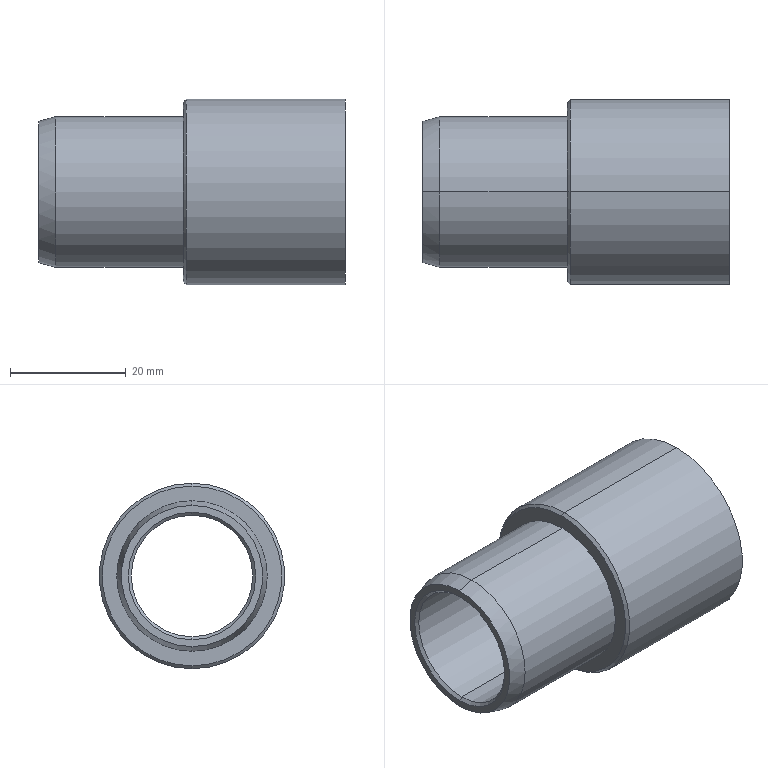Part | SolidWorks | features Chamfer 1, Revolution 1 | 1 solid | 28 faces | box 53 x 32 x 32 mm | volume 15205 mm3 | cylinder 12 | cone 10 | plane 6 | commonest cylinder face diameters 26 x6 21 x2 27.2 x2 32 x2
STEP:
#1=CARTESIAN_POINT('',(-28.114,0.,-10.5));
#2=VERTEX_POINT('',#1);
#3=CARTESIAN_POINT('',(-28.114,0.,10.5));
#4=VERTEX_POINT('',#3);
#5=CARTESIAN_POINT('',(-28.114,0.,0.));
#6=DIRECTION('',(-1.,0.,0.));
#7=DIRECTION('',(0.,0.,-1.));
#8=AXIS2_PLACEMENT_3D('',#5,#6,#7);
#9=CIRCLE('',#8,10.5);
#10=EDGE_CURVE('',#2,#4,#9,.T.);
#11=ORIENTED_EDGE('',*,*,#10,.F.);
#12=CARTESIAN_POINT('',(-28.614,0.,-11.));
#13=VERTEX_POINT('',#12);
#14=CARTESIAN_POINT('',(-28.114,0.,-10.5));
#15=DIRECTION('',(-0.7071,0.,-0.7071));
#16=VECTOR('',#15,1000.);
#17=LINE('',#14,#16);
#18=EDGE_CURVE('',#2,#13,#17,.T.);
#19=ORIENTED_EDGE('',*,*,#18,.T.);
#20=CARTESIAN_POINT('',(-28.614,0.,11.));
#21=VERTEX_POINT('',#20);
#22=CARTESIAN_POINT('',(-28.614,0.,0.));
#23=DIRECTION('',(1.,0.,0.));
#24=DIRECTION('',(0.,0.,-1.));
#25=AXIS2_PLACEMENT_3D('',#22,#23,#24);
#26=CIRCLE('',#25,11.);
#27=EDGE_CURVE('',#21,#13,#26,.T.);
#28=ORIENTED_EDGE('',*,*,#27,.F.);
#29=CARTESIAN_POINT('',(-28.114,0.,10.5));
#30=DIRECTION('',(-0.7071,0.,0.7071));
#31=VECTOR('',#30,1000.);
#32=LINE('',#29,#31);
#33=EDGE_CURVE('',#4,#21,#32,.T.);
#34=ORIENTED_EDGE('',*,*,#33,.F.);
#35=EDGE_LOOP('',(#11,#19,#28,#34));
#36=FACE_OUTER_BOUND('',#35,.T.);
#37=CARTESIAN_POINT('',(-28.114,0.,0.));
#38=DIRECTION('',(-1.,0.,0.));
#39=DIRECTION('',(0.,0.,1.));
#40=AXIS2_PLACEMENT_3D('',#37,#38,#39);
#41=CONICAL_SURFACE('',#40,10.5,0.7854);
#42=ADVANCED_FACE('',(#36),#41,.F.);
#43=CARTESIAN_POINT('',(12.886,0.,10.5));
#44=VERTEX_POINT('',#43);
#45=CARTESIAN_POINT('',(12.886,0.,-10.5));
#46=VERTEX_POINT('',#45);
#47=CARTESIAN_POINT('',(12.886,0.,0.));
#48=DIRECTION('',(1.,0.,0.));
#49=DIRECTION('',(0.,0.,1.));
#50=AXIS2_PLACEMENT_3D('',#47,#48,#49);
#51=CIRCLE('',#50,10.5);
#52=EDGE_CURVE('',#44,#46,#51,.T.);
#53=ORIENTED_EDGE('',*,*,#52,.F.);
#54=CARTESIAN_POINT('',(13.386,0.,11.));
#55=VERTEX_POINT('',#54);
#56=CARTESIAN_POINT('',(13.386,0.,11.));
#57=DIRECTION('',(0.7071,0.,0.7071));
#58=VECTOR('',#57,1000.);
#59=LINE('',#56,#58);
#60=EDGE_CURVE('',#44,#55,#59,.T.);
#61=ORIENTED_EDGE('',*,*,#60,.T.);
#62=CARTESIAN_POINT('',(13.386,0.,-11.));
#63=VERTEX_POINT('',#62);
#64=CARTESIAN_POINT('',(13.386,0.,0.));
#65=DIRECTION('',(-1.,0.,0.));
#66=DIRECTION('',(0.,0.,1.));
#67=AXIS2_PLACEMENT_3D('',#64,#65,#66);
#68=CIRCLE('',#67,11.);
#69=EDGE_CURVE('',#63,#55,#68,.T.);
#70=ORIENTED_EDGE('',*,*,#69,.F.);
#71=CARTESIAN_POINT('',(13.386,0.,-11.));
#72=DIRECTION('',(0.7071,0.,-0.7071));
#73=VECTOR('',#72,1000.);
#74=LINE('',#71,#73);
#75=EDGE_CURVE('',#46,#63,#74,.T.);
#76=ORIENTED_EDGE('',*,*,#75,.F.);
#77=EDGE_LOOP('',(#53,#61,#70,#76));
#78=FACE_OUTER_BOUND('',#77,.T.);
#79=CARTESIAN_POINT('',(13.386,0.,0.));
#80=DIRECTION('',(1.,0.,0.));
#81=DIRECTION('',(0.,0.,-1.));
#82=AXIS2_PLACEMENT_3D('',#79,#80,#81);
#83=CONICAL_SURFACE('',#82,11.,0.7854);
#84=ADVANCED_FACE('',(#78),#83,.F.);
#85=CARTESIAN_POINT('',(23.886,0.,13.));
#86=VERTEX_POINT('',#85);
#87=CARTESIAN_POINT('',(23.886,0.,-13.));
#88=VERTEX_POINT('',#87);
#89=CARTESIAN_POINT('',(23.886,0.,0.));
#90=DIRECTION('',(1.,0.,0.));
#91=DIRECTION('',(0.,0.,1.));
#92=AXIS2_PLACEMENT_3D('',#89,#90,#91);
#93=CIRCLE('',#92,13.);
#94=EDGE_CURVE('',#86,#88,#93,.T.);
#95=ORIENTED_EDGE('',*,*,#94,.F.);
#96=CARTESIAN_POINT('',(24.386,0.,13.5));
#97=VERTEX_POINT('',#96);
#98=CARTESIAN_POINT('',(24.386,0.,13.5));
#99=DIRECTION('',(0.7071,0.,0.7071));
#100=VECTOR('',#99,1000.);
#101=LINE('',#98,#100);
#102=EDGE_CURVE('',#86,#97,#101,.T.);
#103=ORIENTED_EDGE('',*,*,#102,.T.);
#104=CARTESIAN_POINT('',(24.386,0.,-13.5));
#105=VERTEX_POINT('',#104);
#106=CARTESIAN_POINT('',(24.386,0.,0.));
#107=DIRECTION('',(-1.,0.,0.));
#108=DIRECTION('',(0.,0.,1.));
#109=AXIS2_PLACEMENT_3D('',#106,#107,#108);
#110=CIRCLE('',#109,13.5);
#111=EDGE_CURVE('',#105,#97,#110,.T.);
#112=ORIENTED_EDGE('',*,*,#111,.F.);
#113=CARTESIAN_POINT('',(24.386,0.,-13.5));
#114=DIRECTION('',(0.7071,0.,-0.7071));
#115=VECTOR('',#114,1000.);
#116=LINE('',#113,#115);
#117=EDGE_CURVE('',#88,#105,#116,.T.);
#118=ORIENTED_EDGE('',*,*,#117,.F.);
#119=EDGE_LOOP('',(#95,#103,#112,#118));
#120=FACE_OUTER_BOUND('',#119,.T.);
#121=CARTESIAN_POINT('',(24.386,0.,0.));
#122=DIRECTION('',(1.,0.,0.));
#123=DIRECTION('',(0.,0.,-1.));
#124=AXIS2_PLACEMENT_3D('',#121,#122,#123);
#125=CONICAL_SURFACE('',#124,13.5,0.7854);
#126=ADVANCED_FACE('',(#120),#125,.F.);
#127=CARTESIAN_POINT('',(-3.614,0.,15.5));
#128=VERTEX_POINT('',#127);
#129=CARTESIAN_POINT('',(-3.614,0.,-15.5));
#130=VERTEX_POINT('',#129);
#131=CARTESIAN_POINT('',(-3.614,0.,0.));
#132=DIRECTION('',(-1.,0.,0.));
#133=DIRECTION('',(0.,0.,-1.));
#134=AXIS2_PLACEMENT_3D('',#131,#132,#133);
#135=CIRCLE('',#134,15.5);
#136=EDGE_CURVE('',#128,#130,#135,.T.);
#137=ORIENTED_EDGE('',*,*,#136,.F.);
#138=CARTESIAN_POINT('',(-3.114,0.,16.));
#139=VERTEX_POINT('',#138);
#140=CARTESIAN_POINT('',(-3.614,0.,15.5));
#141=DIRECTION('',(0.7071,0.,0.7071));
#142=VECTOR('',#141,1000.);
#143=LINE('',#140,#142);
#144=EDGE_CURVE('',#128,#139,#143,.T.);
#145=ORIENTED_EDGE('',*,*,#144,.T.);
#146=CARTESIAN_POINT('',(-3.114,0.,-16.));
#147=VERTEX_POINT('',#146);
#148=CARTESIAN_POINT('',(-3.114,0.,0.));
#149=DIRECTION('',(1.,0.,0.));
#150=DIRECTION('',(0.,0.,-1.));
#151=AXIS2_PLACEMENT_3D('',#148,#149,#150);
#152=CIRCLE('',#151,16.);
#153=EDGE_CURVE('',#147,#139,#152,.T.);
#154=ORIENTED_EDGE('',*,*,#153,.F.);
#155=CARTESIAN_POINT('',(-3.614,0.,-15.5));
#156=DIRECTION('',(0.7071,0.,-0.7071));
#157=VECTOR('',#156,1000.);
#158=LINE('',#155,#157);
#159=EDGE_CURVE('',#130,#147,#158,.T.);
#160=ORIENTED_EDGE('',*,*,#159,.F.);
#161=EDGE_LOOP('',(#137,#145,#154,#160));
#162=FACE_OUTER_BOUND('',#161,.T.);
#163=CARTESIAN_POINT('',(-3.614,0.,0.));
#164=DIRECTION('',(1.,0.,0.));
#165=DIRECTION('',(0.,0.,-1.));
#166=AXIS2_PLACEMENT_3D('',#163,#164,#165);
#167=CONICAL_SURFACE('',#166,15.5,0.7854);
#168=ADVANCED_FACE('',(#162),#167,.T.);
#169=CARTESIAN_POINT('',(-28.614,0.,12.2));
#170=VERTEX_POINT('',#169);
#171=CARTESIAN_POINT('',(-28.614,0.,-12.2));
#172=VERTEX_POINT('',#171);
#173=CARTESIAN_POINT('',(-28.614,0.,0.));
#174=DIRECTION('',(-1.,0.,0.));
#175=DIRECTION('',(0.,0.,1.));
#176=AXIS2_PLACEMENT_3D('',#173,#174,#175);
#177=CIRCLE('',#176,12.2);
#178=EDGE_CURVE('',#170,#172,#177,.T.);
#179=ORIENTED_EDGE('',*,*,#178,.F.);
#180=CARTESIAN_POINT('',(-25.629,0.,13.));
#181=VERTEX_POINT('',#180);
#182=CARTESIAN_POINT('',(-25.629,0.,13.));
#183=DIRECTION('',(0.9659,0.,0.2588));
#184=VECTOR('',#183,1000.);
#185=LINE('',#182,#184);
#186=EDGE_CURVE('',#170,#181,#185,.T.);
#187=ORIENTED_EDGE('',*,*,#186,.T.);
#188=CARTESIAN_POINT('',(-25.629,0.,-13.));
#189=VERTEX_POINT('',#188);
#190=CARTESIAN_POINT('',(-25.629,0.,0.));
#191=DIRECTION('',(-1.,0.,0.));
#192=DIRECTION('',(0.,0.,1.));
#193=AXIS2_PLACEMENT_3D('',#190,#191,#192);
#194=CIRCLE('',#193,13.);
#195=EDGE_CURVE('',#181,#189,#194,.T.);
#196=ORIENTED_EDGE('',*,*,#195,.T.);
#197=CARTESIAN_POINT('',(-25.629,0.,-13.));
#198=DIRECTION('',(0.9659,0.,-0.2588));
#199=VECTOR('',#198,1000.);
#200=LINE('',#197,#199);
#201=EDGE_CURVE('',#172,#189,#200,.T.);
#202=ORIENTED_EDGE('',*,*,#201,.F.);
#203=EDGE_LOOP('',(#179,#187,#196,#202));
#204=FACE_OUTER_BOUND('',#203,.T.);
#205=CARTESIAN_POINT('',(-25.629,0.,0.));
#206=DIRECTION('',(1.,0.,0.));
#207=DIRECTION('',(0.,0.,-1.));
#208=AXIS2_PLACEMENT_3D('',#205,#206,#207);
#209=CONICAL_SURFACE('',#208,13.,0.2618);
#210=ADVANCED_FACE('',(#204),#209,.T.);
#211=CARTESIAN_POINT('',(-3.614,0.,13.));
#212=VERTEX_POINT('',#211);
#213=CARTESIAN_POINT('',(-3.614,0.,-13.));
#214=VERTEX_POINT('',#213);
#215=CARTESIAN_POINT('',(-3.614,0.,0.));
#216=DIRECTION('',(-1.,0.,0.));
#217=DIRECTION('',(0.,0.,1.));
#218=AXIS2_PLACEMENT_3D('',#215,#216,#217);
#219=CIRCLE('',#218,13.);
#220=EDGE_CURVE('',#212,#214,#219,.T.);
#221=ORIENTED_EDGE('',*,*,#220,.T.);
#222=CARTESIAN_POINT('',(0.,0.,-13.));
#223=DIRECTION('',(-1.,0.,0.));
#224=VECTOR('',#223,1000.);
#225=LINE('',#222,#224);
#226=EDGE_CURVE('',#214,#189,#225,.T.);
#227=ORIENTED_EDGE('',*,*,#226,.T.);
#228=ORIENTED_EDGE('',*,*,#195,.F.);
#229=CARTESIAN_POINT('',(0.,0.,13.));
#230=DIRECTION('',(-1.,0.,0.));
#231=VECTOR('',#230,1000.);
#232=LINE('',#229,#231);
#233=EDGE_CURVE('',#212,#181,#232,.T.);
#234=ORIENTED_EDGE('',*,*,#233,.F.);
#235=EDGE_LOOP('',(#221,#227,#228,#234));
#236=FACE_OUTER_BOUND('',#235,.T.);
#237=CARTESIAN_POINT('',(0.,0.,0.));
#238=DIRECTION('',(-1.,0.,0.));
#239=DIRECTION('',(0.,0.,1.));
#240=AXIS2_PLACEMENT_3D('',#237,#238,#239);
#241=CYLINDRICAL_SURFACE('',#240,13.);
#242=ADVANCED_FACE('',(#236),#241,.T.);
#243=CARTESIAN_POINT('',(24.386,0.,16.));
#244=VERTEX_POINT('',#243);
#245=CARTESIAN_POINT('',(24.386,0.,-16.));
#246=VERTEX_POINT('',#245);
#247=CARTESIAN_POINT('',(24.386,0.,0.));
#248=DIRECTION('',(-1.,0.,0.));
#249=DIRECTION('',(0.,0.,1.));
#250=AXIS2_PLACEMENT_3D('',#247,#248,#249);
#251=CIRCLE('',#250,16.);
#252=EDGE_CURVE('',#244,#246,#251,.T.);
#253=ORIENTED_EDGE('',*,*,#252,.T.);
#254=CARTESIAN_POINT('',(0.,0.,-16.));
#255=DIRECTION('',(-1.,0.,0.));
#256=VECTOR('',#255,1000.);
#257=LINE('',#254,#256);
#258=EDGE_CURVE('',#246,#147,#257,.T.);
#259=ORIENTED_EDGE('',*,*,#258,.T.);
#260=ORIENTED_EDGE('',*,*,#153,.T.);
#261=CARTESIAN_POINT('',(0.,0.,16.));
#262=DIRECTION('',(-1.,0.,0.));
#263=VECTOR('',#262,1000.);
#264=LINE('',#261,#263);
#265=EDGE_CURVE('',#244,#139,#264,.T.);
#266=ORIENTED_EDGE('',*,*,#265,.F.);
#267=EDGE_LOOP('',(#253,#259,#260,#266));
#268=FACE_OUTER_BOUND('',#267,.T.);
#269=CARTESIAN_POINT('',(0.,0.,0.));
#270=DIRECTION('',(-1.,0.,0.));
#271=DIRECTION('',(0.,0.,1.));
#272=AXIS2_PLACEMENT_3D('',#269,#270,#271);
#273=CYLINDRICAL_SURFACE('',#272,16.);
#274=ADVANCED_FACE('',(#268),#273,.T.);
#275=ORIENTED_EDGE('',*,*,#94,.T.);
#276=CARTESIAN_POINT('',(22.686,0.,-13.));
#277=VERTEX_POINT('',#276);
#278=CARTESIAN_POINT('',(0.,0.,-13.));
#279=DIRECTION('',(-1.,0.,0.));
#280=VECTOR('',#279,1000.);
#281=LINE('',#278,#280);
#282=EDGE_CURVE('',#88,#277,#281,.T.);
#283=ORIENTED_EDGE('',*,*,#282,.T.);
#284=CARTESIAN_POINT('',(22.686,0.,13.));
#285=VERTEX_POINT('',#284);
#286=CARTESIAN_POINT('',(22.686,0.,0.));
#287=DIRECTION('',(-1.,0.,0.));
#288=DIRECTION('',(0.,0.,1.));
#289=AXIS2_PLACEMENT_3D('',#286,#287,#288);
#290=CIRCLE('',#289,13.);
#291=EDGE_CURVE('',#277,#285,#290,.T.);
#292=ORIENTED_EDGE('',*,*,#291,.T.);
#293=CARTESIAN_POINT('',(0.,0.,13.));
#294=DIRECTION('',(-1.,0.,0.));
#295=VECTOR('',#294,1000.);
#296=LINE('',#293,#295);
#297=EDGE_CURVE('',#86,#285,#296,.T.);
#298=ORIENTED_EDGE('',*,*,#297,.F.);
#299=EDGE_LOOP('',(#275,#283,#292,#298));
#300=FACE_OUTER_BOUND('',#299,.T.);
#301=CARTESIAN_POINT('',(0.,0.,0.));
#302=DIRECTION('',(-1.,0.,0.));
#303=DIRECTION('',(0.,0.,1.));
#304=AXIS2_PLACEMENT_3D('',#301,#302,#303);
#305=CYLINDRICAL_SURFACE('',#304,13.);
#306=ADVANCED_FACE('',(#300),#305,.F.);
#307=CARTESIAN_POINT('',(22.686,0.,-13.6));
#308=VERTEX_POINT('',#307);
#309=CARTESIAN_POINT('',(22.686,0.,13.6));
#310=VERTEX_POINT('',#309);
#311=CARTESIAN_POINT('',(22.686,0.,0.));
#312=DIRECTION('',(-1.,0.,0.));
#313=DIRECTION('',(0.,0.,1.));
#314=AXIS2_PLACEMENT_3D('',#311,#312,#313);
#315=CIRCLE('',#314,13.6);
#316=EDGE_CURVE('',#308,#310,#315,.T.);
#317=ORIENTED_EDGE('',*,*,#316,.F.);
#318=CARTESIAN_POINT('',(21.386,0.,-13.6));
#319=VERTEX_POINT('',#318);
#320=CARTESIAN_POINT('',(0.,0.,-13.6));
#321=DIRECTION('',(-1.,0.,0.));
#322=VECTOR('',#321,1000.);
#323=LINE('',#320,#322);
#324=EDGE_CURVE('',#308,#319,#323,.T.);
#325=ORIENTED_EDGE('',*,*,#324,.T.);
#326=CARTESIAN_POINT('',(21.386,0.,13.6));
#327=VERTEX_POINT('',#326);
#328=CARTESIAN_POINT('',(21.386,0.,0.));
#329=DIRECTION('',(-1.,0.,0.));
#330=DIRECTION('',(0.,0.,1.));
#331=AXIS2_PLACEMENT_3D('',#328,#329,#330);
#332=CIRCLE('',#331,13.6);
#333=EDGE_CURVE('',#319,#327,#332,.T.);
#334=ORIENTED_EDGE('',*,*,#333,.T.);
#335=CARTESIAN_POINT('',(0.,0.,13.6));
#336=DIRECTION('',(-1.,0.,0.));
#337=VECTOR('',#336,1000.);
#338=LINE('',#335,#337);
#339=EDGE_CURVE('',#310,#327,#338,.T.);
#340=ORIENTED_EDGE('',*,*,#339,.F.);
#341=EDGE_LOOP('',(#317,#325,#334,#340));
#342=FACE_OUTER_BOUND('',#341,.T.);
#343=CARTESIAN_POINT('',(0.,0.,0.));
#344=DIRECTION('',(-1.,0.,0.));
#345=DIRECTION('',(0.,0.,1.));
#346=AXIS2_PLACEMENT_3D('',#343,#344,#345);
#347=CYLINDRICAL_SURFACE('',#346,13.6);
#348=ADVANCED_FACE('',(#342),#347,.F.);
#349=CARTESIAN_POINT('',(21.386,0.,-13.));
#350=VERTEX_POINT('',#349);
#351=CARTESIAN_POINT('',(21.386,0.,13.));
#352=VERTEX_POINT('',#351);
#353=CARTESIAN_POINT('',(21.386,0.,0.));
#354=DIRECTION('',(-1.,0.,0.));
#355=DIRECTION('',(0.,0.,1.));
#356=AXIS2_PLACEMENT_3D('',#353,#354,#355);
#357=CIRCLE('',#356,13.);
#358=EDGE_CURVE('',#350,#352,#357,.T.);
#359=ORIENTED_EDGE('',*,*,#358,.F.);
#360=CARTESIAN_POINT('',(13.386,0.,-13.));
#361=VERTEX_POINT('',#360);
#362=CARTESIAN_POINT('',(0.,0.,-13.));
#363=DIRECTION('',(-1.,0.,0.));
#364=VECTOR('',#363,1000.);
#365=LINE('',#362,#364);
#366=EDGE_CURVE('',#350,#361,#365,.T.);
#367=ORIENTED_EDGE('',*,*,#366,.T.);
#368=CARTESIAN_POINT('',(13.386,0.,13.));
#369=VERTEX_POINT('',#368);
#370=CARTESIAN_POINT('',(13.386,0.,0.));
#371=DIRECTION('',(-1.,0.,0.));
#372=DIRECTION('',(0.,0.,1.));
#373=AXIS2_PLACEMENT_3D('',#370,#371,#372);
#374=CIRCLE('',#373,13.);
#375=EDGE_CURVE('',#361,#369,#374,.T.);
#376=ORIENTED_EDGE('',*,*,#375,.T.);
#377=CARTESIAN_POINT('',(0.,0.,13.));
#378=DIRECTION('',(-1.,0.,0.));
#379=VECTOR('',#378,1000.);
#380=LINE('',#377,#379);
#381=EDGE_CURVE('',#352,#369,#380,.T.);
#382=ORIENTED_EDGE('',*,*,#381,.F.);
#383=EDGE_LOOP('',(#359,#367,#376,#382));
#384=FACE_OUTER_BOUND('',#383,.T.);
#385=CARTESIAN_POINT('',(0.,0.,0.));
#386=DIRECTION('',(-1.,0.,0.));
#387=DIRECTION('',(0.,0.,1.));
#388=AXIS2_PLACEMENT_3D('',#385,#386,#387);
#389=CYLINDRICAL_SURFACE('',#388,13.);
#390=ADVANCED_FACE('',(#384),#389,.F.);
#391=ORIENTED_EDGE('',*,*,#52,.T.);
#392=CARTESIAN_POINT('',(0.,0.,-10.5));
#393=DIRECTION('',(-1.,0.,0.));
#394=VECTOR('',#393,1000.);
#395=LINE('',#392,#394);
#396=EDGE_CURVE('',#46,#2,#395,.T.);
#397=ORIENTED_EDGE('',*,*,#396,.T.);
#398=ORIENTED_EDGE('',*,*,#10,.T.);
#399=CARTESIAN_POINT('',(0.,0.,10.5));
#400=DIRECTION('',(-1.,0.,0.));
#401=VECTOR('',#400,1000.);
#402=LINE('',#399,#401);
#403=EDGE_CURVE('',#44,#4,#402,.T.);
#404=ORIENTED_EDGE('',*,*,#403,.F.);
#405=EDGE_LOOP('',(#391,#397,#398,#404));
#406=FACE_OUTER_BOUND('',#405,.T.);
#407=CARTESIAN_POINT('',(0.,0.,0.));
#408=DIRECTION('',(-1.,0.,0.));
#409=DIRECTION('',(0.,0.,1.));
#410=AXIS2_PLACEMENT_3D('',#407,#408,#409);
#411=CYLINDRICAL_SURFACE('',#410,10.5);
#412=ADVANCED_FACE('',(#406),#411,.F.);
#413=ORIENTED_EDGE('',*,*,#27,.T.);
#414=CARTESIAN_POINT('',(-28.614,0.,0.));
#415=DIRECTION('',(1.,0.,0.));
#416=DIRECTION('',(0.,0.,-1.));
#417=AXIS2_PLACEMENT_3D('',#414,#415,#416);
#418=CIRCLE('',#417,11.);
#419=EDGE_CURVE('',#13,#21,#418,.T.);
#420=ORIENTED_EDGE('',*,*,#419,.T.);
#421=EDGE_LOOP('',(#413,#420));
#422=FACE_BOUND('',#421,.T.);
#423=CARTESIAN_POINT('',(-28.614,0.,0.));
#424=DIRECTION('',(-1.,0.,0.));
#425=DIRECTION('',(0.,0.,1.));
#426=AXIS2_PLACEMENT_3D('',#423,#424,#425);
#427=CIRCLE('',#426,12.2);
#428=EDGE_CURVE('',#172,#170,#427,.T.);
#429=ORIENTED_EDGE('',*,*,#428,.T.);
#430=ORIENTED_EDGE('',*,*,#178,.T.);
#431=EDGE_LOOP('',(#429,#430));
#432=FACE_OUTER_BOUND('',#431,.T.);
#433=CARTESIAN_POINT('',(-28.614,0.,-12.2));
#434=DIRECTION('',(1.,0.,0.));
#435=DIRECTION('',(0.,0.,-1.));
#436=AXIS2_PLACEMENT_3D('',#433,#434,#435);
#437=PLANE('',#436);
#438=ADVANCED_FACE('',(#422,#432),#437,.F.);
#439=ORIENTED_EDGE('',*,*,#396,.F.);
#440=CARTESIAN_POINT('',(12.886,0.,0.));
#441=DIRECTION('',(1.,0.,0.));
#442=DIRECTION('',(0.,0.,1.));
#443=AXIS2_PLACEMENT_3D('',#440,#441,#442);
#444=CIRCLE('',#443,10.5);
#445=EDGE_CURVE('',#46,#44,#444,.T.);
#446=ORIENTED_EDGE('',*,*,#445,.T.);
#447=ORIENTED_EDGE('',*,*,#403,.T.);
#448=CARTESIAN_POINT('',(-28.114,0.,0.));
#449=DIRECTION('',(-1.,0.,0.));
#450=DIRECTION('',(0.,0.,-1.));
#451=AXIS2_PLACEMENT_3D('',#448,#449,#450);
#452=CIRCLE('',#451,10.5);
#453=EDGE_CURVE('',#4,#2,#452,.T.);
#454=ORIENTED_EDGE('',*,*,#453,.T.);
#455=EDGE_LOOP('',(#439,#446,#447,#454));
#456=FACE_OUTER_BOUND('',#455,.T.);
#457=CARTESIAN_POINT('',(0.,0.,0.));
#458=DIRECTION('',(-1.,0.,0.));
#459=DIRECTION('',(0.,0.,1.));
#460=AXIS2_PLACEMENT_3D('',#457,#458,#459);
#461=CYLINDRICAL_SURFACE('',#460,10.5);
#462=ADVANCED_FACE('',(#456),#461,.F.);
#463=ORIENTED_EDGE('',*,*,#69,.T.);
#464=CARTESIAN_POINT('',(13.386,0.,0.));
#465=DIRECTION('',(-1.,0.,0.));
#466=DIRECTION('',(0.,0.,1.));
#467=AXIS2_PLACEMENT_3D('',#464,#465,#466);
#468=CIRCLE('',#467,11.);
#469=EDGE_CURVE('',#55,#63,#468,.T.);
#470=ORIENTED_EDGE('',*,*,#469,.T.);
#471=EDGE_LOOP('',(#463,#470));
#472=FACE_BOUND('',#471,.T.);
#473=CARTESIAN_POINT('',(13.386,0.,0.));
#474=DIRECTION('',(-1.,0.,0.));
#475=DIRECTION('',(0.,0.,1.));
#476=AXIS2_PLACEMENT_3D('',#473,#474,#475);
#477=CIRCLE('',#476,13.);
#478=EDGE_CURVE('',#369,#361,#477,.T.);
#479=ORIENTED_EDGE('',*,*,#478,.F.);
#480=ORIENTED_EDGE('',*,*,#375,.F.);
#481=EDGE_LOOP('',(#479,#480));
#482=FACE_OUTER_BOUND('',#481,.T.);
#483=CARTESIAN_POINT('',(13.386,0.,-10.5));
#484=DIRECTION('',(-1.,0.,0.));
#485=DIRECTION('',(0.,0.,1.));
#486=AXIS2_PLACEMENT_3D('',#483,#484,#485);
#487=PLANE('',#486);
#488=ADVANCED_FACE('',(#472,#482),#487,.F.);
#489=ORIENTED_EDGE('',*,*,#366,.F.);
#490=CARTESIAN_POINT('',(21.386,0.,0.));
#491=DIRECTION('',(-1.,0.,0.));
#492=DIRECTION('',(0.,0.,1.));
#493=AXIS2_PLACEMENT_3D('',#490,#491,#492);
#494=CIRCLE('',#493,13.);
#495=EDGE_CURVE('',#352,#350,#494,.T.);
#496=ORIENTED_EDGE('',*,*,#495,.F.);
#497=ORIENTED_EDGE('',*,*,#381,.T.);
#498=ORIENTED_EDGE('',*,*,#478,.T.);
#499=EDGE_LOOP('',(#489,#496,#497,#498));
#500=FACE_OUTER_BOUND('',#499,.T.);
#501=CARTESIAN_POINT('',(0.,0.,0.));
#502=DIRECTION('',(-1.,0.,0.));
#503=DIRECTION('',(0.,0.,1.));
#504=AXIS2_PLACEMENT_3D('',#501,#502,#503);
#505=CYLINDRICAL_SURFACE('',#504,13.);
#506=ADVANCED_FACE('',(#500),#505,.F.);
#507=CARTESIAN_POINT('',(21.386,0.,0.));
#508=DIRECTION('',(-1.,0.,0.));
#509=DIRECTION('',(0.,0.,1.));
#510=AXIS2_PLACEMENT_3D('',#507,#508,#509);
#511=CIRCLE('',#510,13.6);
#512=EDGE_CURVE('',#327,#319,#511,.T.);
#513=ORIENTED_EDGE('',*,*,#512,.F.);
#514=ORIENTED_EDGE('',*,*,#333,.F.);
#515=EDGE_LOOP('',(#513,#514));
#516=FACE_OUTER_BOUND('',#515,.T.);
#517=ORIENTED_EDGE('',*,*,#495,.T.);
#518=ORIENTED_EDGE('',*,*,#358,.T.);
#519=EDGE_LOOP('',(#517,#518));
#520=FACE_BOUND('',#519,.T.);
#521=CARTESIAN_POINT('',(21.386,0.,-13.));
#522=DIRECTION('',(-1.,0.,0.));
#523=DIRECTION('',(0.,0.,1.));
#524=AXIS2_PLACEMENT_3D('',#521,#522,#523);
#525=PLANE('',#524);
#526=ADVANCED_FACE('',(#516,#520),#525,.F.);
#527=ORIENTED_EDGE('',*,*,#324,.F.);
#528=CARTESIAN_POINT('',(22.686,0.,0.));
#529=DIRECTION('',(-1.,0.,0.));
#530=DIRECTION('',(0.,0.,1.));
#531=AXIS2_PLACEMENT_3D('',#528,#529,#530);
#532=CIRCLE('',#531,13.6);
#533=EDGE_CURVE('',#310,#308,#532,.T.);
#534=ORIENTED_EDGE('',*,*,#533,.F.);
#535=ORIENTED_EDGE('',*,*,#339,.T.);
#536=ORIENTED_EDGE('',*,*,#512,.T.);
#537=EDGE_LOOP('',(#527,#534,#535,#536));
#538=FACE_OUTER_BOUND('',#537,.T.);
#539=CARTESIAN_POINT('',(0.,0.,0.));
#540=DIRECTION('',(-1.,0.,0.));
#541=DIRECTION('',(0.,0.,1.));
#542=AXIS2_PLACEMENT_3D('',#539,#540,#541);
#543=CYLINDRICAL_SURFACE('',#542,13.6);
#544=ADVANCED_FACE('',(#538),#543,.F.);
#545=CARTESIAN_POINT('',(22.686,0.,0.));
#546=DIRECTION('',(-1.,0.,0.));
#547=DIRECTION('',(0.,0.,1.));
#548=AXIS2_PLACEMENT_3D('',#545,#546,#547);
#549=CIRCLE('',#548,13.);
#550=EDGE_CURVE('',#285,#277,#549,.T.);
#551=ORIENTED_EDGE('',*,*,#550,.F.);
#552=ORIENTED_EDGE('',*,*,#291,.F.);
#553=EDGE_LOOP('',(#551,#552));
#554=FACE_BOUND('',#553,.T.);
#555=ORIENTED_EDGE('',*,*,#533,.T.);
#556=ORIENTED_EDGE('',*,*,#316,.T.);
#557=EDGE_LOOP('',(#555,#556));
#558=FACE_OUTER_BOUND('',#557,.T.);
#559=CARTESIAN_POINT('',(22.686,0.,-13.6));
#560=DIRECTION('',(1.,0.,0.));
#561=DIRECTION('',(0.,0.,-1.));
#562=AXIS2_PLACEMENT_3D('',#559,#560,#561);
#563=PLANE('',#562);
#564=ADVANCED_FACE('',(#554,#558),#563,.F.);
#565=ORIENTED_EDGE('',*,*,#282,.F.);
#566=CARTESIAN_POINT('',(23.886,0.,0.));
#567=DIRECTION('',(1.,0.,0.));
#568=DIRECTION('',(0.,0.,1.));
#569=AXIS2_PLACEMENT_3D('',#566,#567,#568);
#570=CIRCLE('',#569,13.);
#571=EDGE_CURVE('',#88,#86,#570,.T.);
#572=ORIENTED_EDGE('',*,*,#571,.T.);
#573=ORIENTED_EDGE('',*,*,#297,.T.);
#574=ORIENTED_EDGE('',*,*,#550,.T.);
#575=EDGE_LOOP('',(#565,#572,#573,#574));
#576=FACE_OUTER_BOUND('',#575,.T.);
#577=CARTESIAN_POINT('',(0.,0.,0.));
#578=DIRECTION('',(-1.,0.,0.));
#579=DIRECTION('',(0.,0.,1.));
#580=AXIS2_PLACEMENT_3D('',#577,#578,#579);
#581=CYLINDRICAL_SURFACE('',#580,13.);
#582=ADVANCED_FACE('',(#576),#581,.F.);
#583=ORIENTED_EDGE('',*,*,#111,.T.);
#584=CARTESIAN_POINT('',(24.386,0.,0.));
#585=DIRECTION('',(-1.,0.,0.));
#586=DIRECTION('',(0.,0.,1.));
#587=AXIS2_PLACEMENT_3D('',#584,#585,#586);
#588=CIRCLE('',#587,13.5);
#589=EDGE_CURVE('',#97,#105,#588,.T.);
#590=ORIENTED_EDGE('',*,*,#589,.T.);
#591=EDGE_LOOP('',(#583,#590));
#592=FACE_BOUND('',#591,.T.);
#593=ORIENTED_EDGE('',*,*,#252,.F.);
#594=CARTESIAN_POINT('',(24.386,0.,0.));
#595=DIRECTION('',(-1.,0.,0.));
#596=DIRECTION('',(0.,0.,1.));
#597=AXIS2_PLACEMENT_3D('',#594,#595,#596);
#598=CIRCLE('',#597,16.);
#599=EDGE_CURVE('',#246,#244,#598,.T.);
#600=ORIENTED_EDGE('',*,*,#599,.F.);
#601=EDGE_LOOP('',(#593,#600));
#602=FACE_OUTER_BOUND('',#601,.T.);
#603=CARTESIAN_POINT('',(24.386,0.,-13.));
#604=DIRECTION('',(-1.,0.,0.));
#605=DIRECTION('',(0.,0.,1.));
#606=AXIS2_PLACEMENT_3D('',#603,#604,#605);
#607=PLANE('',#606);
#608=ADVANCED_FACE('',(#592,#602),#607,.F.);
#609=ORIENTED_EDGE('',*,*,#258,.F.);
#610=ORIENTED_EDGE('',*,*,#599,.T.);
#611=ORIENTED_EDGE('',*,*,#265,.T.);
#612=CARTESIAN_POINT('',(-3.114,0.,0.));
#613=DIRECTION('',(1.,0.,0.));
#614=DIRECTION('',(0.,0.,-1.));
#615=AXIS2_PLACEMENT_3D('',#612,#613,#614);
#616=CIRCLE('',#615,16.);
#617=EDGE_CURVE('',#139,#147,#616,.T.);
#618=ORIENTED_EDGE('',*,*,#617,.T.);
#619=EDGE_LOOP('',(#609,#610,#611,#618));
#620=FACE_OUTER_BOUND('',#619,.T.);
#621=CARTESIAN_POINT('',(0.,0.,0.));
#622=DIRECTION('',(-1.,0.,0.));
#623=DIRECTION('',(0.,0.,1.));
#624=AXIS2_PLACEMENT_3D('',#621,#622,#623);
#625=CYLINDRICAL_SURFACE('',#624,16.);
#626=ADVANCED_FACE('',(#620),#625,.T.);
#627=CARTESIAN_POINT('',(-3.614,0.,0.));
#628=DIRECTION('',(-1.,0.,0.));
#629=DIRECTION('',(0.,0.,-1.));
#630=AXIS2_PLACEMENT_3D('',#627,#628,#629);
#631=CIRCLE('',#630,15.5);
#632=EDGE_CURVE('',#130,#128,#631,.T.);
#633=ORIENTED_EDGE('',*,*,#632,.T.);
#634=ORIENTED_EDGE('',*,*,#136,.T.);
#635=EDGE_LOOP('',(#633,#634));
#636=FACE_OUTER_BOUND('',#635,.T.);
#637=ORIENTED_EDGE('',*,*,#220,.F.);
#638=CARTESIAN_POINT('',(-3.614,0.,0.));
#639=DIRECTION('',(-1.,0.,0.));
#640=DIRECTION('',(0.,0.,1.));
#641=AXIS2_PLACEMENT_3D('',#638,#639,#640);
#642=CIRCLE('',#641,13.);
#643=EDGE_CURVE('',#214,#212,#642,.T.);
#644=ORIENTED_EDGE('',*,*,#643,.F.);
#645=EDGE_LOOP('',(#637,#644));
#646=FACE_BOUND('',#645,.T.);
#647=CARTESIAN_POINT('',(-3.614,0.,-16.));
#648=DIRECTION('',(1.,0.,0.));
#649=DIRECTION('',(0.,0.,-1.));
#650=AXIS2_PLACEMENT_3D('',#647,#648,#649);
#651=PLANE('',#650);
#652=ADVANCED_FACE('',(#636,#646),#651,.F.);
#653=ORIENTED_EDGE('',*,*,#226,.F.);
#654=ORIENTED_EDGE('',*,*,#643,.T.);
#655=ORIENTED_EDGE('',*,*,#233,.T.);
#656=CARTESIAN_POINT('',(-25.629,0.,0.));
#657=DIRECTION('',(-1.,0.,0.));
#658=DIRECTION('',(0.,0.,1.));
#659=AXIS2_PLACEMENT_3D('',#656,#657,#658);
#660=CIRCLE('',#659,13.);
#661=EDGE_CURVE('',#189,#181,#660,.T.);
#662=ORIENTED_EDGE('',*,*,#661,.F.);
#663=EDGE_LOOP('',(#653,#654,#655,#662));
#664=FACE_OUTER_BOUND('',#663,.T.);
#665=CARTESIAN_POINT('',(0.,0.,0.));
#666=DIRECTION('',(-1.,0.,0.));
#667=DIRECTION('',(0.,0.,1.));
#668=AXIS2_PLACEMENT_3D('',#665,#666,#667);
#669=CYLINDRICAL_SURFACE('',#668,13.);
#670=ADVANCED_FACE('',(#664),#669,.T.);
#671=ORIENTED_EDGE('',*,*,#186,.F.);
#672=ORIENTED_EDGE('',*,*,#428,.F.);
#673=ORIENTED_EDGE('',*,*,#201,.T.);
#674=ORIENTED_EDGE('',*,*,#661,.T.);
#675=EDGE_LOOP('',(#671,#672,#673,#674));
#676=FACE_OUTER_BOUND('',#675,.T.);
#677=CARTESIAN_POINT('',(-25.629,0.,0.));
#678=DIRECTION('',(1.,0.,0.));
#679=DIRECTION('',(0.,0.,-1.));
#680=AXIS2_PLACEMENT_3D('',#677,#678,#679);
#681=CONICAL_SURFACE('',#680,13.,0.2618);
#682=ADVANCED_FACE('',(#676),#681,.T.);
#683=ORIENTED_EDGE('',*,*,#144,.F.);
#684=ORIENTED_EDGE('',*,*,#632,.F.);
#685=ORIENTED_EDGE('',*,*,#159,.T.);
#686=ORIENTED_EDGE('',*,*,#617,.F.);
#687=EDGE_LOOP('',(#683,#684,#685,#686));
#688=FACE_OUTER_BOUND('',#687,.T.);
#689=CARTESIAN_POINT('',(-3.614,0.,0.));
#690=DIRECTION('',(1.,0.,0.));
#691=DIRECTION('',(0.,0.,-1.));
#692=AXIS2_PLACEMENT_3D('',#689,#690,#691);
#693=CONICAL_SURFACE('',#692,15.5,0.7854);
#694=ADVANCED_FACE('',(#688),#693,.T.);
#695=ORIENTED_EDGE('',*,*,#102,.F.);
#696=ORIENTED_EDGE('',*,*,#571,.F.);
#697=ORIENTED_EDGE('',*,*,#117,.T.);
#698=ORIENTED_EDGE('',*,*,#589,.F.);
#699=EDGE_LOOP('',(#695,#696,#697,#698));
#700=FACE_OUTER_BOUND('',#699,.T.);
#701=CARTESIAN_POINT('',(24.386,0.,0.));
#702=DIRECTION('',(1.,0.,0.));
#703=DIRECTION('',(0.,0.,-1.));
#704=AXIS2_PLACEMENT_3D('',#701,#702,#703);
#705=CONICAL_SURFACE('',#704,13.5,0.7854);
#706=ADVANCED_FACE('',(#700),#705,.F.);
#707=ORIENTED_EDGE('',*,*,#60,.F.);
#708=ORIENTED_EDGE('',*,*,#445,.F.);
#709=ORIENTED_EDGE('',*,*,#75,.T.);
#710=ORIENTED_EDGE('',*,*,#469,.F.);
#711=EDGE_LOOP('',(#707,#708,#709,#710));
#712=FACE_OUTER_BOUND('',#711,.T.);
#713=CARTESIAN_POINT('',(13.386,0.,0.));
#714=DIRECTION('',(1.,0.,0.));
#715=DIRECTION('',(0.,0.,-1.));
#716=AXIS2_PLACEMENT_3D('',#713,#714,#715);
#717=CONICAL_SURFACE('',#716,11.,0.7854);
#718=ADVANCED_FACE('',(#712),#717,.F.);
#719=ORIENTED_EDGE('',*,*,#18,.F.);
#720=ORIENTED_EDGE('',*,*,#453,.F.);
#721=ORIENTED_EDGE('',*,*,#33,.T.);
#722=ORIENTED_EDGE('',*,*,#419,.F.);
#723=EDGE_LOOP('',(#719,#720,#721,#722));
#724=FACE_OUTER_BOUND('',#723,.T.);
#725=CARTESIAN_POINT('',(-28.114,0.,0.));
#726=DIRECTION('',(-1.,0.,0.));
#727=DIRECTION('',(0.,0.,1.));
#728=AXIS2_PLACEMENT_3D('',#725,#726,#727);
#729=CONICAL_SURFACE('',#728,10.5,0.7854);
#730=ADVANCED_FACE('',(#724),#729,.F.);
#731=CLOSED_SHELL('',(#42,#84,#126,#168,#210,#242,#274,#306,#348,#390,#412,#438,#462,#488,#506,#526,#544,#564,#582,#608,#626,#652,#670,#682,#694,#706,#718,#730));
#732=MANIFOLD_SOLID_BREP('',#731);
#733=CARTESIAN_POINT('',(0.,0.,0.));
#734=DIRECTION('',(0.,0.,1.));
#735=DIRECTION('',(1.,0.,0.));
#736=AXIS2_PLACEMENT_3D('',#733,#734,#735);
#737=(LENGTH_UNIT()NAMED_UNIT(*)SI_UNIT(.MILLI.,.METRE.));
#738=UNCERTAINTY_MEASURE_WITH_UNIT(LENGTH_MEASURE(0.00001),#737,'','');
#739=(NAMED_UNIT(*)PLANE_ANGLE_UNIT()SI_UNIT($,.RADIAN.));
#740=(NAMED_UNIT(*)SI_UNIT($,.STERADIAN.)SOLID_ANGLE_UNIT());
#741=(GEOMETRIC_REPRESENTATION_CONTEXT(3)GLOBAL_UNCERTAINTY_ASSIGNED_CONTEXT((#738))GLOBAL_UNIT_ASSIGNED_CONTEXT((#737,#739,#740))REPRESENTATION_CONTEXT('',''));
#742=ADVANCED_BREP_SHAPE_REPRESENTATION('',(#732,#736),#741);